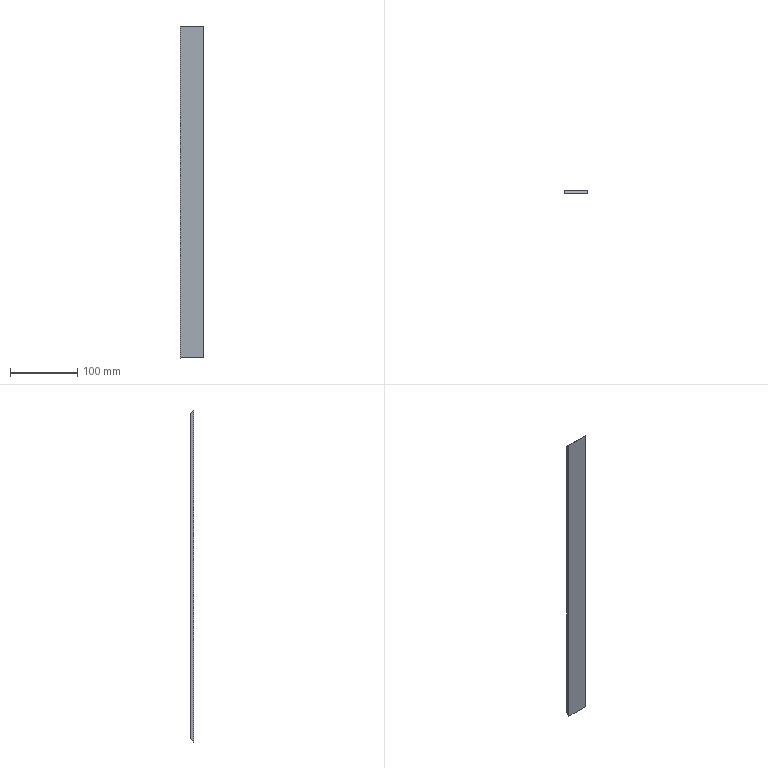Part | STEP file | 09-26 Cover side plate 2 | 1 solid | 6 faces | box 35 x 5 x 495 mm | volume 85750 mm3 | plane 6
STEP:
#1=CARTESIAN_POINT('',(0.,0.,0.));
#2=DIRECTION('',(0.,0.,1.));
#3=DIRECTION('',(1.,0.,0.));
#4=AXIS2_PLACEMENT_3D('',#1,#2,#3);
#5=CARTESIAN_POINT('',(35.,0.,-495.));
#6=VERTEX_POINT('',#5);
#7=CARTESIAN_POINT('',(0.,0.,-495.));
#8=VERTEX_POINT('',#7);
#9=CARTESIAN_POINT('',(17.5,0.,-495.));
#10=DIRECTION('',(-1.,0.,0.));
#11=VECTOR('',#10,1.);
#12=LINE('',#9,#11);
#13=CARTESIAN_POINT('',(0.,0.,-495.));
#14=DIRECTION('',(0.,1.,0.));
#15=DIRECTION('',(0.,0.,1.));
#16=AXIS2_PLACEMENT_3D('',#13,#14,#15);
#17=PLANE('',#16);
#18=CARTESIAN_POINT('',(0.,17.5));
#19=DIRECTION('',(0.,-1.));
#20=VECTOR('',#19,1.);
#21=LINE('',#18,#20);
#22=(GEOMETRIC_REPRESENTATION_CONTEXT(2)PARAMETRIC_REPRESENTATION_CONTEXT()REPRESENTATION_CONTEXT('',''));
#23=DEFINITIONAL_REPRESENTATION('',(#21),#22);
#24=PCURVE('',#17,#23);
#25=CARTESIAN_POINT('',(0.,5.,-490.));
#26=DIRECTION('',(0.,-0.7071,0.7071));
#27=DIRECTION('',(0.,-0.7071,-0.7071));
#28=AXIS2_PLACEMENT_3D('',#25,#26,#27);
#29=PLANE('',#28);
#30=CARTESIAN_POINT('',(7.071,17.5));
#31=DIRECTION('',(0.,-1.));
#32=VECTOR('',#31,1.);
#33=LINE('',#30,#32);
#34=(GEOMETRIC_REPRESENTATION_CONTEXT(2)PARAMETRIC_REPRESENTATION_CONTEXT()REPRESENTATION_CONTEXT('',''));
#35=DEFINITIONAL_REPRESENTATION('',(#33),#34);
#36=PCURVE('',#29,#35);
#37=SURFACE_CURVE('',#12,(#24,#36),.PCURVE_S1.);
#38=EDGE_CURVE('',#6,#8,#37,.T.);
#39=ORIENTED_EDGE('',*,*,#38,.F.);
#40=CARTESIAN_POINT('',(35.,0.,-0.000000061));
#41=VERTEX_POINT('',#40);
#42=CARTESIAN_POINT('',(35.,0.,-247.5));
#43=DIRECTION('',(0.,0.,-1.));
#44=VECTOR('',#43,1.);
#45=LINE('',#42,#44);
#46=CARTESIAN_POINT('',(247.5,35.));
#47=DIRECTION('',(-1.,0.));
#48=VECTOR('',#47,1.);
#49=LINE('',#46,#48);
#50=(GEOMETRIC_REPRESENTATION_CONTEXT(2)PARAMETRIC_REPRESENTATION_CONTEXT()REPRESENTATION_CONTEXT('',''));
#51=DEFINITIONAL_REPRESENTATION('',(#49),#50);
#52=PCURVE('',#17,#51);
#53=CARTESIAN_POINT('',(35.,0.,2.97));
#54=DIRECTION('',(1.,0.,0.));
#55=DIRECTION('',(0.,0.,-1.));
#56=AXIS2_PLACEMENT_3D('',#53,#54,#55);
#57=PLANE('',#56);
#58=CARTESIAN_POINT('',(250.47,0.));
#59=DIRECTION('',(1.,0.));
#60=VECTOR('',#59,1.);
#61=LINE('',#58,#60);
#62=(GEOMETRIC_REPRESENTATION_CONTEXT(2)PARAMETRIC_REPRESENTATION_CONTEXT()REPRESENTATION_CONTEXT('',''));
#63=DEFINITIONAL_REPRESENTATION('',(#61),#62);
#64=PCURVE('',#57,#63);
#65=SURFACE_CURVE('',#45,(#52,#64),.PCURVE_S1.);
#66=EDGE_CURVE('',#41,#6,#65,.T.);
#67=ORIENTED_EDGE('',*,*,#66,.F.);
#68=CARTESIAN_POINT('',(0.,0.,0.));
#69=VERTEX_POINT('',#68);
#70=CARTESIAN_POINT('',(17.5,0.,0.));
#71=DIRECTION('',(1.,0.,0.));
#72=VECTOR('',#71,1.);
#73=LINE('',#70,#72);
#74=CARTESIAN_POINT('',(495.,17.5));
#75=DIRECTION('',(0.,1.));
#76=VECTOR('',#75,1.);
#77=LINE('',#74,#76);
#78=(GEOMETRIC_REPRESENTATION_CONTEXT(2)PARAMETRIC_REPRESENTATION_CONTEXT()REPRESENTATION_CONTEXT('',''));
#79=DEFINITIONAL_REPRESENTATION('',(#77),#78);
#80=PCURVE('',#17,#79);
#81=CARTESIAN_POINT('',(0.,0.,0.));
#82=DIRECTION('',(0.,-0.7071,-0.7071));
#83=DIRECTION('',(0.,0.7071,-0.7071));
#84=AXIS2_PLACEMENT_3D('',#81,#82,#83);
#85=PLANE('',#84);
#86=CARTESIAN_POINT('',(0.,17.5));
#87=DIRECTION('',(0.,1.));
#88=VECTOR('',#87,1.);
#89=LINE('',#86,#88);
#90=(GEOMETRIC_REPRESENTATION_CONTEXT(2)PARAMETRIC_REPRESENTATION_CONTEXT()REPRESENTATION_CONTEXT('',''));
#91=DEFINITIONAL_REPRESENTATION('',(#89),#90);
#92=PCURVE('',#85,#91);
#93=SURFACE_CURVE('',#73,(#80,#92),.PCURVE_S1.);
#94=EDGE_CURVE('',#69,#41,#93,.T.);
#95=ORIENTED_EDGE('',*,*,#94,.F.);
#96=CARTESIAN_POINT('',(0.,0.,-247.5));
#97=DIRECTION('',(0.,0.,1.));
#98=VECTOR('',#97,1.);
#99=LINE('',#96,#98);
#100=CARTESIAN_POINT('',(247.5,0.));
#101=DIRECTION('',(1.,0.));
#102=VECTOR('',#101,1.);
#103=LINE('',#100,#102);
#104=(GEOMETRIC_REPRESENTATION_CONTEXT(2)PARAMETRIC_REPRESENTATION_CONTEXT()REPRESENTATION_CONTEXT('',''));
#105=DEFINITIONAL_REPRESENTATION('',(#103),#104);
#106=PCURVE('',#17,#105);
#107=CARTESIAN_POINT('',(0.,0.,2.97));
#108=DIRECTION('',(1.,0.,0.));
#109=DIRECTION('',(0.,0.,-1.));
#110=AXIS2_PLACEMENT_3D('',#107,#108,#109);
#111=PLANE('',#110);
#112=CARTESIAN_POINT('',(250.47,0.));
#113=DIRECTION('',(-1.,0.));
#114=VECTOR('',#113,1.);
#115=LINE('',#112,#114);
#116=(GEOMETRIC_REPRESENTATION_CONTEXT(2)PARAMETRIC_REPRESENTATION_CONTEXT()REPRESENTATION_CONTEXT('',''));
#117=DEFINITIONAL_REPRESENTATION('',(#115),#116);
#118=PCURVE('',#111,#117);
#119=SURFACE_CURVE('',#99,(#106,#118),.PCURVE_S1.);
#120=EDGE_CURVE('',#8,#69,#119,.T.);
#121=ORIENTED_EDGE('',*,*,#120,.F.);
#122=EDGE_LOOP('',(#39,#67,#95,#121));
#123=FACE_BOUND('',#122,.T.);
#124=ADVANCED_FACE('',(#123),#17,.F.);
#125=CARTESIAN_POINT('',(0.,5.,-5.));
#126=VERTEX_POINT('',#125);
#127=CARTESIAN_POINT('',(0.,0.,0.));
#128=DIRECTION('',(0.,-0.7071,0.7071));
#129=VECTOR('',#128,1.);
#130=LINE('',#127,#129);
#131=CARTESIAN_POINT('',(2.97,0.));
#132=DIRECTION('',(-0.7071,-0.7071));
#133=VECTOR('',#132,1.);
#134=LINE('',#131,#133);
#135=(GEOMETRIC_REPRESENTATION_CONTEXT(2)PARAMETRIC_REPRESENTATION_CONTEXT()REPRESENTATION_CONTEXT('',''));
#136=DEFINITIONAL_REPRESENTATION('',(#134),#135);
#137=PCURVE('',#111,#136);
#138=CARTESIAN_POINT('',(0.,0.));
#139=DIRECTION('',(-1.,0.));
#140=VECTOR('',#139,1.);
#141=LINE('',#138,#140);
#142=(GEOMETRIC_REPRESENTATION_CONTEXT(2)PARAMETRIC_REPRESENTATION_CONTEXT()REPRESENTATION_CONTEXT('',''));
#143=DEFINITIONAL_REPRESENTATION('',(#141),#142);
#144=PCURVE('',#85,#143);
#145=SURFACE_CURVE('',#130,(#137,#144),.PCURVE_S1.);
#146=EDGE_CURVE('',#126,#69,#145,.T.);
#147=ORIENTED_EDGE('',*,*,#146,.F.);
#148=CARTESIAN_POINT('',(0.,5.,-490.));
#149=VERTEX_POINT('',#148);
#150=CARTESIAN_POINT('',(0.,5.,-247.5));
#151=DIRECTION('',(0.,0.,1.));
#152=VECTOR('',#151,1.);
#153=LINE('',#150,#152);
#154=CARTESIAN_POINT('',(250.47,5.));
#155=DIRECTION('',(-1.,0.));
#156=VECTOR('',#155,1.);
#157=LINE('',#154,#156);
#158=(GEOMETRIC_REPRESENTATION_CONTEXT(2)PARAMETRIC_REPRESENTATION_CONTEXT()REPRESENTATION_CONTEXT('',''));
#159=DEFINITIONAL_REPRESENTATION('',(#157),#158);
#160=PCURVE('',#111,#159);
#161=CARTESIAN_POINT('',(0.,5.,-5.));
#162=DIRECTION('',(0.,-1.,0.));
#163=DIRECTION('',(0.,0.,-1.));
#164=AXIS2_PLACEMENT_3D('',#161,#162,#163);
#165=PLANE('',#164);
#166=CARTESIAN_POINT('',(242.5,0.));
#167=DIRECTION('',(-1.,0.));
#168=VECTOR('',#167,1.);
#169=LINE('',#166,#168);
#170=(GEOMETRIC_REPRESENTATION_CONTEXT(2)PARAMETRIC_REPRESENTATION_CONTEXT()REPRESENTATION_CONTEXT('',''));
#171=DEFINITIONAL_REPRESENTATION('',(#169),#170);
#172=PCURVE('',#165,#171);
#173=SURFACE_CURVE('',#153,(#160,#172),.PCURVE_S1.);
#174=EDGE_CURVE('',#149,#126,#173,.T.);
#175=ORIENTED_EDGE('',*,*,#174,.F.);
#176=CARTESIAN_POINT('',(0.,5.,-490.));
#177=DIRECTION('',(0.,0.7071,0.7071));
#178=VECTOR('',#177,1.);
#179=LINE('',#176,#178);
#180=CARTESIAN_POINT('',(492.97,5.));
#181=DIRECTION('',(-0.7071,0.7071));
#182=VECTOR('',#181,1.);
#183=LINE('',#180,#182);
#184=(GEOMETRIC_REPRESENTATION_CONTEXT(2)PARAMETRIC_REPRESENTATION_CONTEXT()REPRESENTATION_CONTEXT('',''));
#185=DEFINITIONAL_REPRESENTATION('',(#183),#184);
#186=PCURVE('',#111,#185);
#187=CARTESIAN_POINT('',(0.,0.));
#188=DIRECTION('',(-1.,0.));
#189=VECTOR('',#188,1.);
#190=LINE('',#187,#189);
#191=(GEOMETRIC_REPRESENTATION_CONTEXT(2)PARAMETRIC_REPRESENTATION_CONTEXT()REPRESENTATION_CONTEXT('',''));
#192=DEFINITIONAL_REPRESENTATION('',(#190),#191);
#193=PCURVE('',#29,#192);
#194=SURFACE_CURVE('',#179,(#186,#193),.PCURVE_S1.);
#195=EDGE_CURVE('',#8,#149,#194,.T.);
#196=ORIENTED_EDGE('',*,*,#195,.F.);
#197=ORIENTED_EDGE('',*,*,#120,.T.);
#198=EDGE_LOOP('',(#147,#175,#196,#197));
#199=FACE_BOUND('',#198,.T.);
#200=ADVANCED_FACE('',(#199),#111,.F.);
#201=CARTESIAN_POINT('',(35.,5.,-490.));
#202=VERTEX_POINT('',#201);
#203=CARTESIAN_POINT('',(17.5,5.,-490.));
#204=DIRECTION('',(-1.,0.,0.));
#205=VECTOR('',#204,1.);
#206=LINE('',#203,#205);
#207=CARTESIAN_POINT('',(0.,17.5));
#208=DIRECTION('',(0.,-1.));
#209=VECTOR('',#208,1.);
#210=LINE('',#207,#209);
#211=(GEOMETRIC_REPRESENTATION_CONTEXT(2)PARAMETRIC_REPRESENTATION_CONTEXT()REPRESENTATION_CONTEXT('',''));
#212=DEFINITIONAL_REPRESENTATION('',(#210),#211);
#213=PCURVE('',#29,#212);
#214=CARTESIAN_POINT('',(485.,17.5));
#215=DIRECTION('',(0.,-1.));
#216=VECTOR('',#215,1.);
#217=LINE('',#214,#216);
#218=(GEOMETRIC_REPRESENTATION_CONTEXT(2)PARAMETRIC_REPRESENTATION_CONTEXT()REPRESENTATION_CONTEXT('',''));
#219=DEFINITIONAL_REPRESENTATION('',(#217),#218);
#220=PCURVE('',#165,#219);
#221=SURFACE_CURVE('',#206,(#213,#220),.PCURVE_S1.);
#222=EDGE_CURVE('',#202,#149,#221,.T.);
#223=ORIENTED_EDGE('',*,*,#222,.F.);
#224=CARTESIAN_POINT('',(35.,2.5,-492.5));
#225=DIRECTION('',(0.,0.7071,0.7071));
#226=VECTOR('',#225,1.);
#227=LINE('',#224,#226);
#228=CARTESIAN_POINT('',(3.536,35.));
#229=DIRECTION('',(-1.,0.));
#230=VECTOR('',#229,1.);
#231=LINE('',#228,#230);
#232=(GEOMETRIC_REPRESENTATION_CONTEXT(2)PARAMETRIC_REPRESENTATION_CONTEXT()REPRESENTATION_CONTEXT('',''));
#233=DEFINITIONAL_REPRESENTATION('',(#231),#232);
#234=PCURVE('',#29,#233);
#235=CARTESIAN_POINT('',(495.47,2.5));
#236=DIRECTION('',(-0.7071,0.7071));
#237=VECTOR('',#236,1.);
#238=LINE('',#235,#237);
#239=(GEOMETRIC_REPRESENTATION_CONTEXT(2)PARAMETRIC_REPRESENTATION_CONTEXT()REPRESENTATION_CONTEXT('',''));
#240=DEFINITIONAL_REPRESENTATION('',(#238),#239);
#241=PCURVE('',#57,#240);
#242=SURFACE_CURVE('',#227,(#234,#241),.PCURVE_S1.);
#243=EDGE_CURVE('',#6,#202,#242,.T.);
#244=ORIENTED_EDGE('',*,*,#243,.F.);
#245=ORIENTED_EDGE('',*,*,#38,.T.);
#246=ORIENTED_EDGE('',*,*,#195,.T.);
#247=EDGE_LOOP('',(#223,#244,#245,#246));
#248=FACE_BOUND('',#247,.T.);
#249=ADVANCED_FACE('',(#248),#29,.F.);
#250=CARTESIAN_POINT('',(35.,5.,-5.));
#251=VERTEX_POINT('',#250);
#252=CARTESIAN_POINT('',(35.,5.,-247.5));
#253=DIRECTION('',(0.,0.,1.));
#254=VECTOR('',#253,1.);
#255=LINE('',#252,#254);
#256=CARTESIAN_POINT('',(250.47,5.));
#257=DIRECTION('',(-1.,0.));
#258=VECTOR('',#257,1.);
#259=LINE('',#256,#258);
#260=(GEOMETRIC_REPRESENTATION_CONTEXT(2)PARAMETRIC_REPRESENTATION_CONTEXT()REPRESENTATION_CONTEXT('',''));
#261=DEFINITIONAL_REPRESENTATION('',(#259),#260);
#262=PCURVE('',#57,#261);
#263=CARTESIAN_POINT('',(242.5,35.));
#264=DIRECTION('',(-1.,0.));
#265=VECTOR('',#264,1.);
#266=LINE('',#263,#265);
#267=(GEOMETRIC_REPRESENTATION_CONTEXT(2)PARAMETRIC_REPRESENTATION_CONTEXT()REPRESENTATION_CONTEXT('',''));
#268=DEFINITIONAL_REPRESENTATION('',(#266),#267);
#269=PCURVE('',#165,#268);
#270=SURFACE_CURVE('',#255,(#262,#269),.PCURVE_S1.);
#271=EDGE_CURVE('',#202,#251,#270,.T.);
#272=ORIENTED_EDGE('',*,*,#271,.T.);
#273=CARTESIAN_POINT('',(35.,5.,-5.));
#274=DIRECTION('',(0.,-0.7071,0.7071));
#275=VECTOR('',#274,1.);
#276=LINE('',#273,#275);
#277=CARTESIAN_POINT('',(7.97,5.));
#278=DIRECTION('',(-0.7071,-0.7071));
#279=VECTOR('',#278,1.);
#280=LINE('',#277,#279);
#281=(GEOMETRIC_REPRESENTATION_CONTEXT(2)PARAMETRIC_REPRESENTATION_CONTEXT()REPRESENTATION_CONTEXT('',''));
#282=DEFINITIONAL_REPRESENTATION('',(#280),#281);
#283=PCURVE('',#57,#282);
#284=CARTESIAN_POINT('',(7.071,35.));
#285=DIRECTION('',(-1.,0.));
#286=VECTOR('',#285,1.);
#287=LINE('',#284,#286);
#288=(GEOMETRIC_REPRESENTATION_CONTEXT(2)PARAMETRIC_REPRESENTATION_CONTEXT()REPRESENTATION_CONTEXT('',''));
#289=DEFINITIONAL_REPRESENTATION('',(#287),#288);
#290=PCURVE('',#85,#289);
#291=SURFACE_CURVE('',#276,(#283,#290),.PCURVE_S1.);
#292=EDGE_CURVE('',#251,#41,#291,.T.);
#293=ORIENTED_EDGE('',*,*,#292,.T.);
#294=ORIENTED_EDGE('',*,*,#66,.T.);
#295=ORIENTED_EDGE('',*,*,#243,.T.);
#296=EDGE_LOOP('',(#272,#293,#294,#295));
#297=FACE_BOUND('',#296,.T.);
#298=ADVANCED_FACE('',(#297),#57,.T.);
#299=ORIENTED_EDGE('',*,*,#94,.T.);
#300=ORIENTED_EDGE('',*,*,#292,.F.);
#301=CARTESIAN_POINT('',(17.5,5.,-5.));
#302=DIRECTION('',(1.,0.,0.));
#303=VECTOR('',#302,1.);
#304=LINE('',#301,#303);
#305=CARTESIAN_POINT('',(7.071,17.5));
#306=DIRECTION('',(0.,1.));
#307=VECTOR('',#306,1.);
#308=LINE('',#305,#307);
#309=(GEOMETRIC_REPRESENTATION_CONTEXT(2)PARAMETRIC_REPRESENTATION_CONTEXT()REPRESENTATION_CONTEXT('',''));
#310=DEFINITIONAL_REPRESENTATION('',(#308),#309);
#311=PCURVE('',#85,#310);
#312=CARTESIAN_POINT('',(0.,17.5));
#313=DIRECTION('',(0.,1.));
#314=VECTOR('',#313,1.);
#315=LINE('',#312,#314);
#316=(GEOMETRIC_REPRESENTATION_CONTEXT(2)PARAMETRIC_REPRESENTATION_CONTEXT()REPRESENTATION_CONTEXT('',''));
#317=DEFINITIONAL_REPRESENTATION('',(#315),#316);
#318=PCURVE('',#165,#317);
#319=SURFACE_CURVE('',#304,(#311,#318),.PCURVE_S1.);
#320=EDGE_CURVE('',#126,#251,#319,.T.);
#321=ORIENTED_EDGE('',*,*,#320,.F.);
#322=ORIENTED_EDGE('',*,*,#146,.T.);
#323=EDGE_LOOP('',(#299,#300,#321,#322));
#324=FACE_BOUND('',#323,.T.);
#325=ADVANCED_FACE('',(#324),#85,.F.);
#326=ORIENTED_EDGE('',*,*,#320,.T.);
#327=ORIENTED_EDGE('',*,*,#271,.F.);
#328=ORIENTED_EDGE('',*,*,#222,.T.);
#329=ORIENTED_EDGE('',*,*,#174,.T.);
#330=EDGE_LOOP('',(#326,#327,#328,#329));
#331=FACE_BOUND('',#330,.T.);
#332=ADVANCED_FACE('',(#331),#165,.F.);
#333=CLOSED_SHELL('',(#124,#200,#249,#298,#325,#332));
#334=MANIFOLD_SOLID_BREP('',#333);
#335=(LENGTH_UNIT()NAMED_UNIT(*)SI_UNIT(.MILLI.,.METRE.));
#336=UNCERTAINTY_MEASURE_WITH_UNIT(LENGTH_MEASURE(0.0000001),#335,'','');
#337=(NAMED_UNIT(*)PLANE_ANGLE_UNIT()SI_UNIT($,.RADIAN.));
#338=(NAMED_UNIT(*)SI_UNIT($,.STERADIAN.)SOLID_ANGLE_UNIT());
#339=(GEOMETRIC_REPRESENTATION_CONTEXT(3)GLOBAL_UNCERTAINTY_ASSIGNED_CONTEXT((#336))GLOBAL_UNIT_ASSIGNED_CONTEXT((#335,#337,#338))REPRESENTATION_CONTEXT('',''));
#340=ADVANCED_BREP_SHAPE_REPRESENTATION('',(#4,#334),#339);